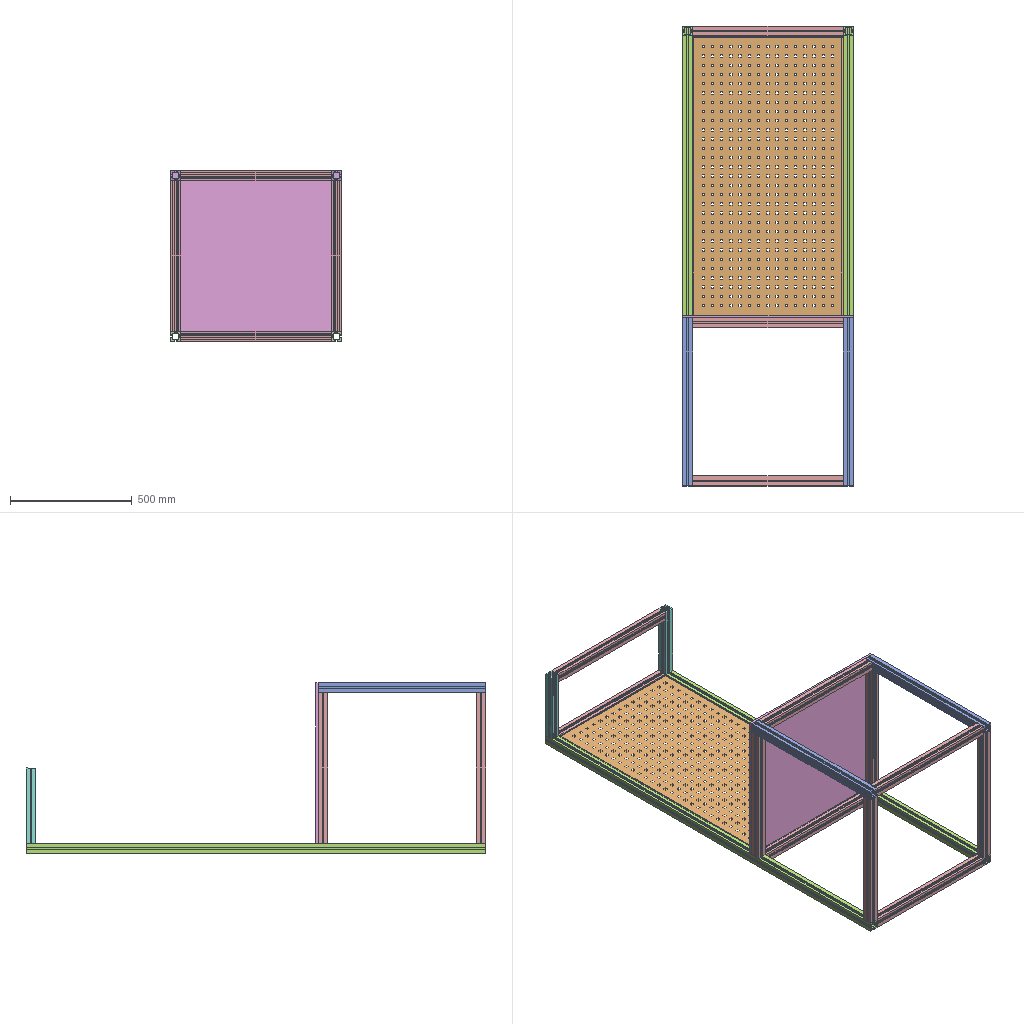Assembly | SolidWorks | 6 different items | 18 placed | box 700 x 1890 x 700 mm
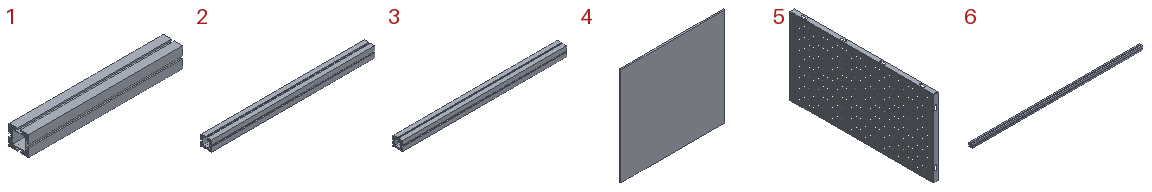Parts list (item | quantity | size | volume | features):
1 | x2 | 310 x 40 x 40 mm | 215760 mm3 | features Extrusion 1
2 | x10 | 620 x 40 x 40 mm | 431520 mm3 | features Extrusion 1
3 | x2 | 690 x 40 x 40 mm | 480240 mm3 | features Extrusion 1
4 | x1 | 700 x 10 x 660 mm | 4620000 mm3 | features Extrusion 1
5 | x1 | 40 x 1158 x 618 mm | 1589634 mm3 | features ICE 3, LPattern 3, EdgeFlange 1, FlatPattern 1, SMBaseFlange 1, SheetMetal 1
6 | x2 | 1890 x 40 x 40 mm | 1315440 mm3 | features Extrusion 1
Mates (type | each side: item.copy, entity, surface, feature):
Coincident | 2.1 face plane Boss-Extrude1 | 3.1 face plane Boss-Extrude1 | 3 times
Coincident | 2.1 face plane Boss-Extrude1 | 3.2 face plane Boss-Extrude1 | 3 times
Coincident | 3.1 face plane Boss-Extrude1 | 2.2 face plane Boss-Extrude1 | 2 times
Coincident | 2.1 face plane Boss-Extrude1 | 2.2 face plane Boss-Extrude1
Coincident | 2.1 face plane Boss-Extrude1 | 2.3 face plane Boss-Extrude1 | 2 times
Coincident | 3.2 face plane Boss-Extrude1 | 2.3 face plane Boss-Extrude1
Coincident | 2.2 face plane Boss-Extrude1 | 6.1 face plane Boss-Extrude1 | 3 times
Coincident | 2.3 face plane Boss-Extrude1 | 6.2 face plane Boss-Extrude1 | 2 times
Coincident | 6.1 face plane Boss-Extrude1 | 6.2 face plane Boss-Extrude1
Coincident | 6.1 face plane Boss-Extrude1 | 2.4 face plane Boss-Extrude1
Coincident | 2.2 face plane Boss-Extrude1 | 2.4 face plane Boss-Extrude1
Coincident | 6.2 face plane Boss-Extrude1 | 2.4 face plane Boss-Extrude1
Coincident | 2.5 face plane Boss-Extrude1 | 4.1 face plane Boss-Extrude1
Coincident | 4.1 face plane Boss-Extrude1 | 6.1 face plane Boss-Extrude1
Coincident | 6.1 face plane Boss-Extrude1 | 4.1 face plane Boss-Extrude1
Coincident | 6.1 face plane Boss-Extrude1 | 2.6 face plane Boss-Extrude1 | 2 times
Coincident | 6.2 face plane Boss-Extrude1 | 2.6 face plane Boss-Extrude1
Coincident | 6.1 face plane Boss-Extrude1 | 1.1 face plane Boss-Extrude1 | 2 times
Coincident | 2.6 face plane Boss-Extrude1 | 1.1 face plane Boss-Extrude1
Coincident | 6.2 face plane Boss-Extrude1 | 1.2 face plane Boss-Extrude1 | 2 times
Coincident | 2.6 face plane Boss-Extrude1 | 1.2 face plane Boss-Extrude1
Coincident | 2.7 face plane Boss-Extrude1 | 1.1 face plane Boss-Extrude1 | 3 times
Coincident | 6.2 face plane Boss-Extrude1 | 5.1 face plane Base-Flange1
Coincident | 6.2 face plane Boss-Extrude1 | 5.1 face plane Edge-Flange1
Coincident | 4.1 face plane Boss-Extrude1 | 5.1 face plane Edge-Flange1